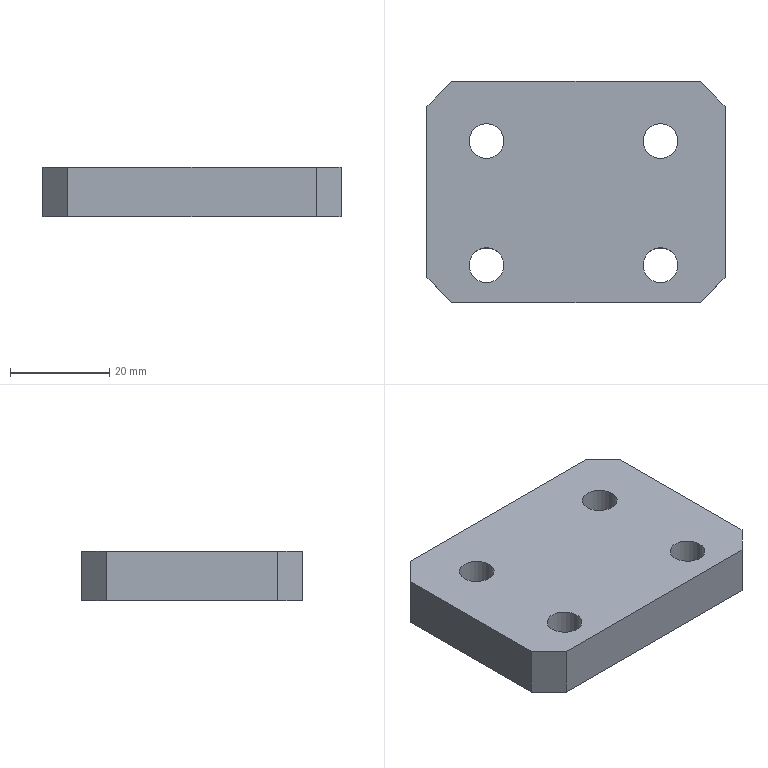Part | NX | features BREP 1 | 1 solid | 14 faces | box 60 x 44.5 x 10 mm | volume 24661 mm3 | plane 10 | cylinder 4 | commonest cylinder face diameters 7 x4
STEP:
#1=CARTESIAN_POINT('',(-30.,-17.25,0.));
#2=VERTEX_POINT('',#1);
#3=CARTESIAN_POINT('',(-25.,-22.25,0.));
#4=VERTEX_POINT('',#3);
#5=CARTESIAN_POINT('',(-30.,-17.25,0.));
#6=DIRECTION('',(0.7071,-0.7071,0.));
#7=VECTOR('',#6,1000.);
#8=LINE('',#5,#7);
#9=EDGE_CURVE('',#2,#4,#8,.T.);
#10=ORIENTED_EDGE('',*,*,#9,.F.);
#11=CARTESIAN_POINT('',(-30.,17.25,0.));
#12=VERTEX_POINT('',#11);
#13=CARTESIAN_POINT('',(-30.,0.,0.));
#14=DIRECTION('',(0.,-1.,0.));
#15=VECTOR('',#14,1000.);
#16=LINE('',#13,#15);
#17=EDGE_CURVE('',#12,#2,#16,.T.);
#18=ORIENTED_EDGE('',*,*,#17,.F.);
#19=CARTESIAN_POINT('',(-25.,22.25,0.));
#20=VERTEX_POINT('',#19);
#21=CARTESIAN_POINT('',(-25.,22.25,0.));
#22=DIRECTION('',(-0.7071,-0.7071,0.));
#23=VECTOR('',#22,1000.);
#24=LINE('',#21,#23);
#25=EDGE_CURVE('',#20,#12,#24,.T.);
#26=ORIENTED_EDGE('',*,*,#25,.F.);
#27=CARTESIAN_POINT('',(25.,22.25,0.));
#28=VERTEX_POINT('',#27);
#29=CARTESIAN_POINT('',(0.,22.25,0.));
#30=DIRECTION('',(-1.,0.,0.));
#31=VECTOR('',#30,1000.);
#32=LINE('',#29,#31);
#33=EDGE_CURVE('',#28,#20,#32,.T.);
#34=ORIENTED_EDGE('',*,*,#33,.F.);
#35=CARTESIAN_POINT('',(30.,17.25,0.));
#36=VERTEX_POINT('',#35);
#37=CARTESIAN_POINT('',(30.,17.25,0.));
#38=DIRECTION('',(-0.7071,0.7071,0.));
#39=VECTOR('',#38,1000.);
#40=LINE('',#37,#39);
#41=EDGE_CURVE('',#36,#28,#40,.T.);
#42=ORIENTED_EDGE('',*,*,#41,.F.);
#43=CARTESIAN_POINT('',(30.,-17.25,0.));
#44=VERTEX_POINT('',#43);
#45=CARTESIAN_POINT('',(30.,0.,0.));
#46=DIRECTION('',(0.,1.,0.));
#47=VECTOR('',#46,1000.);
#48=LINE('',#45,#47);
#49=EDGE_CURVE('',#44,#36,#48,.T.);
#50=ORIENTED_EDGE('',*,*,#49,.F.);
#51=CARTESIAN_POINT('',(25.,-22.25,0.));
#52=VERTEX_POINT('',#51);
#53=CARTESIAN_POINT('',(25.,-22.25,0.));
#54=DIRECTION('',(0.7071,0.7071,0.));
#55=VECTOR('',#54,1000.);
#56=LINE('',#53,#55);
#57=EDGE_CURVE('',#52,#44,#56,.T.);
#58=ORIENTED_EDGE('',*,*,#57,.F.);
#59=CARTESIAN_POINT('',(0.,-22.25,0.));
#60=DIRECTION('',(1.,0.,0.));
#61=VECTOR('',#60,1000.);
#62=LINE('',#59,#61);
#63=EDGE_CURVE('',#4,#52,#62,.T.);
#64=ORIENTED_EDGE('',*,*,#63,.F.);
#65=EDGE_LOOP('',(#10,#18,#26,#34,#42,#50,#58,#64));
#66=FACE_BOUND('',#65,.T.);
#67=CARTESIAN_POINT('',(-14.5,-14.75,0.));
#68=VERTEX_POINT('',#67);
#69=CARTESIAN_POINT('',(-18.,-14.75,0.));
#70=DIRECTION('',(0.,0.,-1.));
#71=DIRECTION('',(1.,0.,0.));
#72=AXIS2_PLACEMENT_3D('',#69,#70,#71);
#73=CIRCLE('',#72,3.5);
#74=EDGE_CURVE('',#68,#68,#73,.T.);
#75=ORIENTED_EDGE('',*,*,#74,.F.);
#76=EDGE_LOOP('',(#75));
#77=FACE_BOUND('',#76,.T.);
#78=CARTESIAN_POINT('',(-14.5,10.25,0.));
#79=VERTEX_POINT('',#78);
#80=CARTESIAN_POINT('',(-18.,10.25,0.));
#81=DIRECTION('',(0.,0.,-1.));
#82=DIRECTION('',(1.,0.,0.));
#83=AXIS2_PLACEMENT_3D('',#80,#81,#82);
#84=CIRCLE('',#83,3.5);
#85=EDGE_CURVE('',#79,#79,#84,.T.);
#86=ORIENTED_EDGE('',*,*,#85,.F.);
#87=EDGE_LOOP('',(#86));
#88=FACE_BOUND('',#87,.T.);
#89=CARTESIAN_POINT('',(20.5,-14.75,0.));
#90=VERTEX_POINT('',#89);
#91=CARTESIAN_POINT('',(17.,-14.75,0.));
#92=DIRECTION('',(0.,0.,-1.));
#93=DIRECTION('',(1.,0.,0.));
#94=AXIS2_PLACEMENT_3D('',#91,#92,#93);
#95=CIRCLE('',#94,3.5);
#96=EDGE_CURVE('',#90,#90,#95,.T.);
#97=ORIENTED_EDGE('',*,*,#96,.F.);
#98=EDGE_LOOP('',(#97));
#99=FACE_BOUND('',#98,.T.);
#100=CARTESIAN_POINT('',(20.5,10.25,0.));
#101=VERTEX_POINT('',#100);
#102=CARTESIAN_POINT('',(17.,10.25,0.));
#103=DIRECTION('',(0.,0.,-1.));
#104=DIRECTION('',(1.,0.,0.));
#105=AXIS2_PLACEMENT_3D('',#102,#103,#104);
#106=CIRCLE('',#105,3.5);
#107=EDGE_CURVE('',#101,#101,#106,.T.);
#108=ORIENTED_EDGE('',*,*,#107,.F.);
#109=EDGE_LOOP('',(#108));
#110=FACE_BOUND('',#109,.T.);
#111=CARTESIAN_POINT('',(0.,0.,0.));
#112=DIRECTION('',(0.,0.,1.));
#113=DIRECTION('',(-1.,0.,0.));
#114=AXIS2_PLACEMENT_3D('',#111,#112,#113);
#115=PLANE('',#114);
#116=ADVANCED_FACE('',(#66,#77,#88,#99,#110),#115,.F.);
#117=CARTESIAN_POINT('',(-25.,-22.25,10.));
#118=VERTEX_POINT('',#117);
#119=CARTESIAN_POINT('',(-25.,-22.25,10.));
#120=DIRECTION('',(0.,0.,1.));
#121=VECTOR('',#120,1000.);
#122=LINE('',#119,#121);
#123=EDGE_CURVE('',#4,#118,#122,.T.);
#124=ORIENTED_EDGE('',*,*,#123,.F.);
#125=ORIENTED_EDGE('',*,*,#63,.T.);
#126=CARTESIAN_POINT('',(25.,-22.25,10.));
#127=VERTEX_POINT('',#126);
#128=CARTESIAN_POINT('',(25.,-22.25,10.));
#129=DIRECTION('',(0.,0.,-1.));
#130=VECTOR('',#129,1000.);
#131=LINE('',#128,#130);
#132=EDGE_CURVE('',#127,#52,#131,.T.);
#133=ORIENTED_EDGE('',*,*,#132,.F.);
#134=CARTESIAN_POINT('',(-30.,-22.25,10.));
#135=DIRECTION('',(1.,0.,0.));
#136=VECTOR('',#135,1000.);
#137=LINE('',#134,#136);
#138=EDGE_CURVE('',#118,#127,#137,.T.);
#139=ORIENTED_EDGE('',*,*,#138,.F.);
#140=EDGE_LOOP('',(#124,#125,#133,#139));
#141=FACE_BOUND('',#140,.T.);
#142=CARTESIAN_POINT('',(-30.,-22.25,10.));
#143=DIRECTION('',(0.,1.,0.));
#144=DIRECTION('',(0.,0.,-1.));
#145=AXIS2_PLACEMENT_3D('',#142,#143,#144);
#146=PLANE('',#145);
#147=ADVANCED_FACE('',(#141),#146,.F.);
#148=CARTESIAN_POINT('',(-30.,-17.25,10.));
#149=VERTEX_POINT('',#148);
#150=CARTESIAN_POINT('',(-30.,-17.25,10.));
#151=DIRECTION('',(0.,0.,1.));
#152=VECTOR('',#151,1000.);
#153=LINE('',#150,#152);
#154=EDGE_CURVE('',#2,#149,#153,.T.);
#155=ORIENTED_EDGE('',*,*,#154,.F.);
#156=ORIENTED_EDGE('',*,*,#9,.T.);
#157=ORIENTED_EDGE('',*,*,#123,.T.);
#158=CARTESIAN_POINT('',(-25.,-22.25,10.));
#159=DIRECTION('',(0.7071,-0.7071,0.));
#160=VECTOR('',#159,1000.);
#161=LINE('',#158,#160);
#162=EDGE_CURVE('',#149,#118,#161,.T.);
#163=ORIENTED_EDGE('',*,*,#162,.F.);
#164=EDGE_LOOP('',(#155,#156,#157,#163));
#165=FACE_BOUND('',#164,.T.);
#166=CARTESIAN_POINT('',(-25.,-22.25,10.));
#167=DIRECTION('',(0.7071,0.7071,0.));
#168=DIRECTION('',(0.7071,-0.7071,0.));
#169=AXIS2_PLACEMENT_3D('',#166,#167,#168);
#170=PLANE('',#169);
#171=ADVANCED_FACE('',(#165),#170,.F.);
#172=ORIENTED_EDGE('',*,*,#154,.T.);
#173=CARTESIAN_POINT('',(-30.,17.25,10.));
#174=VERTEX_POINT('',#173);
#175=CARTESIAN_POINT('',(-30.,22.25,10.));
#176=DIRECTION('',(0.,-1.,0.));
#177=VECTOR('',#176,1000.);
#178=LINE('',#175,#177);
#179=EDGE_CURVE('',#174,#149,#178,.T.);
#180=ORIENTED_EDGE('',*,*,#179,.F.);
#181=CARTESIAN_POINT('',(-30.,17.25,10.));
#182=DIRECTION('',(0.,0.,1.));
#183=VECTOR('',#182,1000.);
#184=LINE('',#181,#183);
#185=EDGE_CURVE('',#12,#174,#184,.T.);
#186=ORIENTED_EDGE('',*,*,#185,.F.);
#187=ORIENTED_EDGE('',*,*,#17,.T.);
#188=EDGE_LOOP('',(#172,#180,#186,#187));
#189=FACE_BOUND('',#188,.T.);
#190=CARTESIAN_POINT('',(-30.,22.25,10.));
#191=DIRECTION('',(1.,0.,0.));
#192=DIRECTION('',(0.,-1.,0.));
#193=AXIS2_PLACEMENT_3D('',#190,#191,#192);
#194=PLANE('',#193);
#195=ADVANCED_FACE('',(#189),#194,.F.);
#196=CARTESIAN_POINT('',(-25.,22.25,10.));
#197=VERTEX_POINT('',#196);
#198=CARTESIAN_POINT('',(-25.,22.25,10.));
#199=DIRECTION('',(0.,0.,1.));
#200=VECTOR('',#199,1000.);
#201=LINE('',#198,#200);
#202=EDGE_CURVE('',#20,#197,#201,.T.);
#203=ORIENTED_EDGE('',*,*,#202,.F.);
#204=ORIENTED_EDGE('',*,*,#25,.T.);
#205=ORIENTED_EDGE('',*,*,#185,.T.);
#206=CARTESIAN_POINT('',(-30.,17.25,10.));
#207=DIRECTION('',(-0.7071,-0.7071,0.));
#208=VECTOR('',#207,1000.);
#209=LINE('',#206,#208);
#210=EDGE_CURVE('',#197,#174,#209,.T.);
#211=ORIENTED_EDGE('',*,*,#210,.F.);
#212=EDGE_LOOP('',(#203,#204,#205,#211));
#213=FACE_BOUND('',#212,.T.);
#214=CARTESIAN_POINT('',(-30.,17.25,10.));
#215=DIRECTION('',(0.7071,-0.7071,0.));
#216=DIRECTION('',(-0.7071,-0.7071,0.));
#217=AXIS2_PLACEMENT_3D('',#214,#215,#216);
#218=PLANE('',#217);
#219=ADVANCED_FACE('',(#213),#218,.F.);
#220=ORIENTED_EDGE('',*,*,#202,.T.);
#221=CARTESIAN_POINT('',(25.,22.25,10.));
#222=VERTEX_POINT('',#221);
#223=CARTESIAN_POINT('',(-30.,22.25,10.));
#224=DIRECTION('',(-1.,0.,0.));
#225=VECTOR('',#224,1000.);
#226=LINE('',#223,#225);
#227=EDGE_CURVE('',#222,#197,#226,.T.);
#228=ORIENTED_EDGE('',*,*,#227,.F.);
#229=CARTESIAN_POINT('',(25.,22.25,10.));
#230=DIRECTION('',(0.,0.,1.));
#231=VECTOR('',#230,1000.);
#232=LINE('',#229,#231);
#233=EDGE_CURVE('',#28,#222,#232,.T.);
#234=ORIENTED_EDGE('',*,*,#233,.F.);
#235=ORIENTED_EDGE('',*,*,#33,.T.);
#236=EDGE_LOOP('',(#220,#228,#234,#235));
#237=FACE_BOUND('',#236,.T.);
#238=CARTESIAN_POINT('',(-30.,22.25,10.));
#239=DIRECTION('',(0.,-1.,0.));
#240=DIRECTION('',(0.,0.,1.));
#241=AXIS2_PLACEMENT_3D('',#238,#239,#240);
#242=PLANE('',#241);
#243=ADVANCED_FACE('',(#237),#242,.F.);
#244=CARTESIAN_POINT('',(30.,17.25,10.));
#245=VERTEX_POINT('',#244);
#246=CARTESIAN_POINT('',(30.,17.25,10.));
#247=DIRECTION('',(0.,0.,1.));
#248=VECTOR('',#247,1000.);
#249=LINE('',#246,#248);
#250=EDGE_CURVE('',#36,#245,#249,.T.);
#251=ORIENTED_EDGE('',*,*,#250,.F.);
#252=ORIENTED_EDGE('',*,*,#41,.T.);
#253=ORIENTED_EDGE('',*,*,#233,.T.);
#254=CARTESIAN_POINT('',(25.,22.25,10.));
#255=DIRECTION('',(-0.7071,0.7071,0.));
#256=VECTOR('',#255,1000.);
#257=LINE('',#254,#256);
#258=EDGE_CURVE('',#245,#222,#257,.T.);
#259=ORIENTED_EDGE('',*,*,#258,.F.);
#260=EDGE_LOOP('',(#251,#252,#253,#259));
#261=FACE_BOUND('',#260,.T.);
#262=CARTESIAN_POINT('',(25.,22.25,10.));
#263=DIRECTION('',(-0.7071,-0.7071,0.));
#264=DIRECTION('',(-0.7071,0.7071,0.));
#265=AXIS2_PLACEMENT_3D('',#262,#263,#264);
#266=PLANE('',#265);
#267=ADVANCED_FACE('',(#261),#266,.F.);
#268=CARTESIAN_POINT('',(30.,-17.25,10.));
#269=VERTEX_POINT('',#268);
#270=CARTESIAN_POINT('',(30.,-17.25,10.));
#271=DIRECTION('',(0.,0.,1.));
#272=VECTOR('',#271,1000.);
#273=LINE('',#270,#272);
#274=EDGE_CURVE('',#44,#269,#273,.T.);
#275=ORIENTED_EDGE('',*,*,#274,.F.);
#276=ORIENTED_EDGE('',*,*,#49,.T.);
#277=ORIENTED_EDGE('',*,*,#250,.T.);
#278=CARTESIAN_POINT('',(30.,22.25,10.));
#279=DIRECTION('',(0.,1.,0.));
#280=VECTOR('',#279,1000.);
#281=LINE('',#278,#280);
#282=EDGE_CURVE('',#269,#245,#281,.T.);
#283=ORIENTED_EDGE('',*,*,#282,.F.);
#284=EDGE_LOOP('',(#275,#276,#277,#283));
#285=FACE_BOUND('',#284,.T.);
#286=CARTESIAN_POINT('',(30.,22.25,10.));
#287=DIRECTION('',(-1.,0.,0.));
#288=DIRECTION('',(0.,1.,0.));
#289=AXIS2_PLACEMENT_3D('',#286,#287,#288);
#290=PLANE('',#289);
#291=ADVANCED_FACE('',(#285),#290,.F.);
#292=ORIENTED_EDGE('',*,*,#132,.T.);
#293=ORIENTED_EDGE('',*,*,#57,.T.);
#294=ORIENTED_EDGE('',*,*,#274,.T.);
#295=CARTESIAN_POINT('',(30.,-17.25,10.));
#296=DIRECTION('',(0.7071,0.7071,0.));
#297=VECTOR('',#296,1000.);
#298=LINE('',#295,#297);
#299=EDGE_CURVE('',#127,#269,#298,.T.);
#300=ORIENTED_EDGE('',*,*,#299,.F.);
#301=EDGE_LOOP('',(#292,#293,#294,#300));
#302=FACE_BOUND('',#301,.T.);
#303=CARTESIAN_POINT('',(30.,-17.25,10.));
#304=DIRECTION('',(-0.7071,0.7071,0.));
#305=DIRECTION('',(0.7071,0.7071,0.));
#306=AXIS2_PLACEMENT_3D('',#303,#304,#305);
#307=PLANE('',#306);
#308=ADVANCED_FACE('',(#302),#307,.F.);
#309=ORIENTED_EDGE('',*,*,#74,.T.);
#310=EDGE_LOOP('',(#309));
#311=FACE_BOUND('',#310,.T.);
#312=CARTESIAN_POINT('',(-14.5,-14.75,10.));
#313=VERTEX_POINT('',#312);
#314=CARTESIAN_POINT('',(-18.,-14.75,10.));
#315=DIRECTION('',(0.,0.,-1.));
#316=DIRECTION('',(1.,0.,0.));
#317=AXIS2_PLACEMENT_3D('',#314,#315,#316);
#318=CIRCLE('',#317,3.5);
#319=EDGE_CURVE('',#313,#313,#318,.T.);
#320=ORIENTED_EDGE('',*,*,#319,.F.);
#321=EDGE_LOOP('',(#320));
#322=FACE_BOUND('',#321,.T.);
#323=CARTESIAN_POINT('',(-18.,-14.75,10.));
#324=DIRECTION('',(0.,0.,1.));
#325=DIRECTION('',(-1.,0.,0.));
#326=AXIS2_PLACEMENT_3D('',#323,#324,#325);
#327=CYLINDRICAL_SURFACE('',#326,3.5);
#328=ADVANCED_FACE('',(#311,#322),#327,.F.);
#329=ORIENTED_EDGE('',*,*,#85,.T.);
#330=EDGE_LOOP('',(#329));
#331=FACE_BOUND('',#330,.T.);
#332=CARTESIAN_POINT('',(-14.5,10.25,10.));
#333=VERTEX_POINT('',#332);
#334=CARTESIAN_POINT('',(-18.,10.25,10.));
#335=DIRECTION('',(0.,0.,-1.));
#336=DIRECTION('',(1.,0.,0.));
#337=AXIS2_PLACEMENT_3D('',#334,#335,#336);
#338=CIRCLE('',#337,3.5);
#339=EDGE_CURVE('',#333,#333,#338,.T.);
#340=ORIENTED_EDGE('',*,*,#339,.F.);
#341=EDGE_LOOP('',(#340));
#342=FACE_BOUND('',#341,.T.);
#343=CARTESIAN_POINT('',(-18.,10.25,10.));
#344=DIRECTION('',(0.,0.,1.));
#345=DIRECTION('',(-1.,0.,0.));
#346=AXIS2_PLACEMENT_3D('',#343,#344,#345);
#347=CYLINDRICAL_SURFACE('',#346,3.5);
#348=ADVANCED_FACE('',(#331,#342),#347,.F.);
#349=ORIENTED_EDGE('',*,*,#96,.T.);
#350=EDGE_LOOP('',(#349));
#351=FACE_BOUND('',#350,.T.);
#352=CARTESIAN_POINT('',(20.5,-14.75,10.));
#353=VERTEX_POINT('',#352);
#354=CARTESIAN_POINT('',(17.,-14.75,10.));
#355=DIRECTION('',(0.,0.,-1.));
#356=DIRECTION('',(1.,0.,0.));
#357=AXIS2_PLACEMENT_3D('',#354,#355,#356);
#358=CIRCLE('',#357,3.5);
#359=EDGE_CURVE('',#353,#353,#358,.T.);
#360=ORIENTED_EDGE('',*,*,#359,.F.);
#361=EDGE_LOOP('',(#360));
#362=FACE_BOUND('',#361,.T.);
#363=CARTESIAN_POINT('',(17.,-14.75,10.));
#364=DIRECTION('',(0.,0.,1.));
#365=DIRECTION('',(-1.,0.,0.));
#366=AXIS2_PLACEMENT_3D('',#363,#364,#365);
#367=CYLINDRICAL_SURFACE('',#366,3.5);
#368=ADVANCED_FACE('',(#351,#362),#367,.F.);
#369=ORIENTED_EDGE('',*,*,#107,.T.);
#370=EDGE_LOOP('',(#369));
#371=FACE_BOUND('',#370,.T.);
#372=CARTESIAN_POINT('',(20.5,10.25,10.));
#373=VERTEX_POINT('',#372);
#374=CARTESIAN_POINT('',(17.,10.25,10.));
#375=DIRECTION('',(0.,0.,-1.));
#376=DIRECTION('',(1.,0.,0.));
#377=AXIS2_PLACEMENT_3D('',#374,#375,#376);
#378=CIRCLE('',#377,3.5);
#379=EDGE_CURVE('',#373,#373,#378,.T.);
#380=ORIENTED_EDGE('',*,*,#379,.F.);
#381=EDGE_LOOP('',(#380));
#382=FACE_BOUND('',#381,.T.);
#383=CARTESIAN_POINT('',(17.,10.25,10.));
#384=DIRECTION('',(0.,0.,1.));
#385=DIRECTION('',(-1.,0.,0.));
#386=AXIS2_PLACEMENT_3D('',#383,#384,#385);
#387=CYLINDRICAL_SURFACE('',#386,3.5);
#388=ADVANCED_FACE('',(#371,#382),#387,.F.);
#389=ORIENTED_EDGE('',*,*,#227,.T.);
#390=ORIENTED_EDGE('',*,*,#210,.T.);
#391=ORIENTED_EDGE('',*,*,#179,.T.);
#392=ORIENTED_EDGE('',*,*,#162,.T.);
#393=ORIENTED_EDGE('',*,*,#138,.T.);
#394=ORIENTED_EDGE('',*,*,#299,.T.);
#395=ORIENTED_EDGE('',*,*,#282,.T.);
#396=ORIENTED_EDGE('',*,*,#258,.T.);
#397=EDGE_LOOP('',(#389,#390,#391,#392,#393,#394,#395,#396));
#398=FACE_BOUND('',#397,.T.);
#399=ORIENTED_EDGE('',*,*,#319,.T.);
#400=EDGE_LOOP('',(#399));
#401=FACE_BOUND('',#400,.T.);
#402=ORIENTED_EDGE('',*,*,#339,.T.);
#403=EDGE_LOOP('',(#402));
#404=FACE_BOUND('',#403,.T.);
#405=ORIENTED_EDGE('',*,*,#359,.T.);
#406=EDGE_LOOP('',(#405));
#407=FACE_BOUND('',#406,.T.);
#408=ORIENTED_EDGE('',*,*,#379,.T.);
#409=EDGE_LOOP('',(#408));
#410=FACE_BOUND('',#409,.T.);
#411=CARTESIAN_POINT('',(0.,0.,10.));
#412=DIRECTION('',(0.,0.,1.));
#413=DIRECTION('',(-1.,0.,0.));
#414=AXIS2_PLACEMENT_3D('',#411,#412,#413);
#415=PLANE('',#414);
#416=ADVANCED_FACE('',(#398,#401,#404,#407,#410),#415,.T.);
#417=CLOSED_SHELL('',(#116,#147,#171,#195,#219,#243,#267,#291,#308,#328,#348,#368,#388,#416));
#418=MANIFOLD_SOLID_BREP('',#417);
#419=(LENGTH_UNIT()NAMED_UNIT(*)SI_UNIT(.MILLI.,.METRE.));
#420=UNCERTAINTY_MEASURE_WITH_UNIT(LENGTH_MEASURE(0.00001),#419,'','');
#421=(NAMED_UNIT(*)PLANE_ANGLE_UNIT()SI_UNIT($,.RADIAN.));
#422=(NAMED_UNIT(*)SI_UNIT($,.STERADIAN.)SOLID_ANGLE_UNIT());
#423=(GEOMETRIC_REPRESENTATION_CONTEXT(3)GLOBAL_UNCERTAINTY_ASSIGNED_CONTEXT((#420))GLOBAL_UNIT_ASSIGNED_CONTEXT((#419,#421,#422))REPRESENTATION_CONTEXT('',''));
#424=ADVANCED_BREP_SHAPE_REPRESENTATION('',(#418),#423);